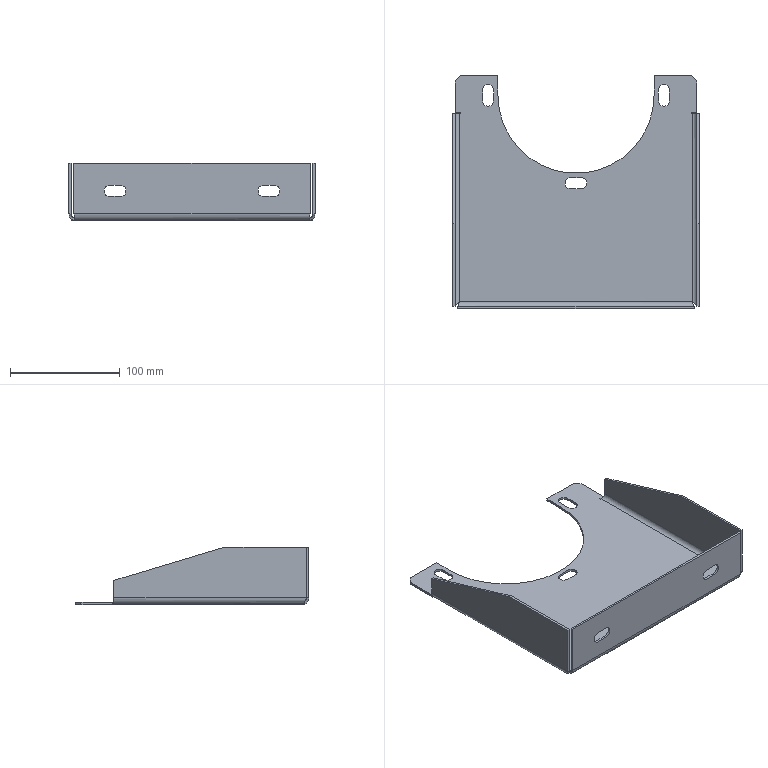Part | STEP file | SYL_0392D6J1SYL0380DJ1006_2_1-1 | 1 solid | 67 faces | box 224 x 212 x 52 mm | volume 119868 mm3 | plane 45 | cylinder 18 | spline 4 | commonest cylinder face diameters 10 x11 8 x3 12 x3 142 x1